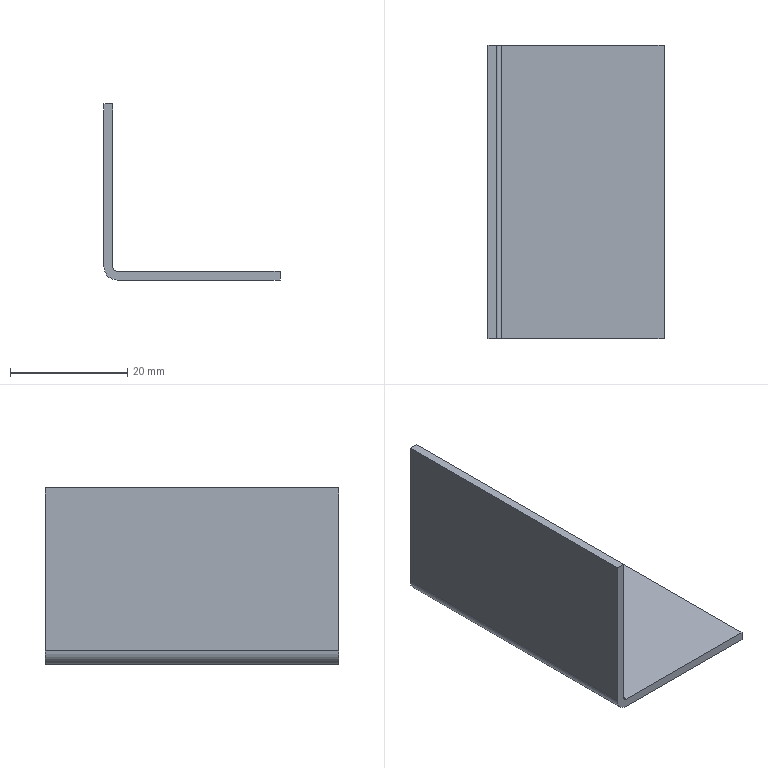Part | 1 solid | 10 faces | box 30 x 50 x 30 mm | volume 4340 mm3 | plane 8 | cylinder 2 | commonest cylinder face diameters 1.473 x1 4.473 x1
STEP:
#1=CARTESIAN_POINT('',(2.237,0.,-28.5));
#2=VERTEX_POINT('',#1);
#3=CARTESIAN_POINT('',(30.,0.,-28.5));
#4=VERTEX_POINT('',#3);
#5=CARTESIAN_POINT('',(0.,0.,-28.5));
#6=DIRECTION('',(1.,0.,0.));
#7=VECTOR('',#6,1000.);
#8=LINE('',#5,#7);
#9=EDGE_CURVE('',#2,#4,#8,.T.);
#10=ORIENTED_EDGE('',*,*,#9,.T.);
#11=CARTESIAN_POINT('',(30.,50.,-28.5));
#12=VERTEX_POINT('',#11);
#13=CARTESIAN_POINT('',(30.,50.,-28.5));
#14=DIRECTION('',(0.,-1.,0.));
#15=VECTOR('',#14,1000.);
#16=LINE('',#13,#15);
#17=EDGE_CURVE('',#12,#4,#16,.T.);
#18=ORIENTED_EDGE('',*,*,#17,.F.);
#19=CARTESIAN_POINT('',(2.237,50.,-28.5));
#20=VERTEX_POINT('',#19);
#21=CARTESIAN_POINT('',(0.,50.,-28.5));
#22=DIRECTION('',(1.,0.,0.));
#23=VECTOR('',#22,1000.);
#24=LINE('',#21,#23);
#25=EDGE_CURVE('',#20,#12,#24,.T.);
#26=ORIENTED_EDGE('',*,*,#25,.F.);
#27=CARTESIAN_POINT('',(2.237,50.,-28.5));
#28=DIRECTION('',(0.,-1.,0.));
#29=VECTOR('',#28,1000.);
#30=LINE('',#27,#29);
#31=EDGE_CURVE('',#20,#2,#30,.T.);
#32=ORIENTED_EDGE('',*,*,#31,.T.);
#33=EDGE_LOOP('',(#10,#18,#26,#32));
#34=FACE_OUTER_BOUND('',#33,.T.);
#35=CARTESIAN_POINT('',(0.,50.,-28.5));
#36=DIRECTION('',(0.,0.,-1.));
#37=DIRECTION('',(-1.,0.,0.));
#38=AXIS2_PLACEMENT_3D('',#35,#36,#37);
#39=PLANE('',#38);
#40=ADVANCED_FACE('',(#34),#39,.F.);
#41=CARTESIAN_POINT('',(30.,0.,-30.));
#42=VERTEX_POINT('',#41);
#43=CARTESIAN_POINT('',(30.,0.,-30.));
#44=DIRECTION('',(0.,0.,1.));
#45=VECTOR('',#44,1000.);
#46=LINE('',#43,#45);
#47=EDGE_CURVE('',#42,#4,#46,.T.);
#48=ORIENTED_EDGE('',*,*,#47,.F.);
#49=CARTESIAN_POINT('',(30.,50.,-30.));
#50=VERTEX_POINT('',#49);
#51=CARTESIAN_POINT('',(30.,50.,-30.));
#52=DIRECTION('',(0.,-1.,0.));
#53=VECTOR('',#52,1000.);
#54=LINE('',#51,#53);
#55=EDGE_CURVE('',#50,#42,#54,.T.);
#56=ORIENTED_EDGE('',*,*,#55,.F.);
#57=CARTESIAN_POINT('',(30.,50.,-30.));
#58=DIRECTION('',(0.,0.,1.));
#59=VECTOR('',#58,1000.);
#60=LINE('',#57,#59);
#61=EDGE_CURVE('',#50,#12,#60,.T.);
#62=ORIENTED_EDGE('',*,*,#61,.T.);
#63=ORIENTED_EDGE('',*,*,#17,.T.);
#64=EDGE_LOOP('',(#48,#56,#62,#63));
#65=FACE_OUTER_BOUND('',#64,.T.);
#66=CARTESIAN_POINT('',(30.,50.,-30.));
#67=DIRECTION('',(1.,0.,0.));
#68=DIRECTION('',(0.,0.,-1.));
#69=AXIS2_PLACEMENT_3D('',#66,#67,#68);
#70=PLANE('',#69);
#71=ADVANCED_FACE('',(#65),#70,.T.);
#72=CARTESIAN_POINT('',(2.237,0.,-30.));
#73=VERTEX_POINT('',#72);
#74=CARTESIAN_POINT('',(0.,0.,-30.));
#75=DIRECTION('',(1.,0.,0.));
#76=VECTOR('',#75,1000.);
#77=LINE('',#74,#76);
#78=EDGE_CURVE('',#73,#42,#77,.T.);
#79=ORIENTED_EDGE('',*,*,#78,.F.);
#80=CARTESIAN_POINT('',(2.237,50.,-30.));
#81=VERTEX_POINT('',#80);
#82=CARTESIAN_POINT('',(2.237,50.,-30.));
#83=DIRECTION('',(0.,-1.,0.));
#84=VECTOR('',#83,1000.);
#85=LINE('',#82,#84);
#86=EDGE_CURVE('',#81,#73,#85,.T.);
#87=ORIENTED_EDGE('',*,*,#86,.F.);
#88=CARTESIAN_POINT('',(0.,50.,-30.));
#89=DIRECTION('',(1.,0.,0.));
#90=VECTOR('',#89,1000.);
#91=LINE('',#88,#90);
#92=EDGE_CURVE('',#81,#50,#91,.T.);
#93=ORIENTED_EDGE('',*,*,#92,.T.);
#94=ORIENTED_EDGE('',*,*,#55,.T.);
#95=EDGE_LOOP('',(#79,#87,#93,#94));
#96=FACE_OUTER_BOUND('',#95,.T.);
#97=CARTESIAN_POINT('',(0.,50.,-30.));
#98=DIRECTION('',(0.,0.,-1.));
#99=DIRECTION('',(-1.,0.,0.));
#100=AXIS2_PLACEMENT_3D('',#97,#98,#99);
#101=PLANE('',#100);
#102=ADVANCED_FACE('',(#96),#101,.T.);
#103=CARTESIAN_POINT('',(0.,0.,-27.763));
#104=VERTEX_POINT('',#103);
#105=CARTESIAN_POINT('',(2.237,0.,-27.763));
#106=DIRECTION('',(0.,-1.,0.));
#107=DIRECTION('',(0.,0.,1.));
#108=AXIS2_PLACEMENT_3D('',#105,#106,#107);
#109=CIRCLE('',#108,2.237);
#110=EDGE_CURVE('',#104,#73,#109,.T.);
#111=ORIENTED_EDGE('',*,*,#110,.F.);
#112=CARTESIAN_POINT('',(0.,50.,-27.763));
#113=VERTEX_POINT('',#112);
#114=CARTESIAN_POINT('',(0.,50.,-27.763));
#115=DIRECTION('',(0.,-1.,0.));
#116=VECTOR('',#115,1000.);
#117=LINE('',#114,#116);
#118=EDGE_CURVE('',#113,#104,#117,.T.);
#119=ORIENTED_EDGE('',*,*,#118,.F.);
#120=CARTESIAN_POINT('',(2.237,50.,-27.763));
#121=DIRECTION('',(0.,-1.,0.));
#122=DIRECTION('',(0.,0.,1.));
#123=AXIS2_PLACEMENT_3D('',#120,#121,#122);
#124=CIRCLE('',#123,2.237);
#125=EDGE_CURVE('',#113,#81,#124,.T.);
#126=ORIENTED_EDGE('',*,*,#125,.T.);
#127=ORIENTED_EDGE('',*,*,#86,.T.);
#128=EDGE_LOOP('',(#111,#119,#126,#127));
#129=FACE_OUTER_BOUND('',#128,.T.);
#130=CARTESIAN_POINT('',(2.237,50.,-27.763));
#131=DIRECTION('',(0.,-1.,0.));
#132=DIRECTION('',(0.,0.,-1.));
#133=AXIS2_PLACEMENT_3D('',#130,#131,#132);
#134=CYLINDRICAL_SURFACE('',#133,2.237);
#135=ADVANCED_FACE('',(#129),#134,.T.);
#136=CARTESIAN_POINT('',(0.,0.,0.));
#137=VERTEX_POINT('',#136);
#138=CARTESIAN_POINT('',(0.,0.,-30.));
#139=DIRECTION('',(0.,0.,-1.));
#140=VECTOR('',#139,1000.);
#141=LINE('',#138,#140);
#142=EDGE_CURVE('',#137,#104,#141,.T.);
#143=ORIENTED_EDGE('',*,*,#142,.F.);
#144=CARTESIAN_POINT('',(0.,50.,0.));
#145=VERTEX_POINT('',#144);
#146=CARTESIAN_POINT('',(0.,50.,0.));
#147=DIRECTION('',(0.,-1.,0.));
#148=VECTOR('',#147,1000.);
#149=LINE('',#146,#148);
#150=EDGE_CURVE('',#145,#137,#149,.T.);
#151=ORIENTED_EDGE('',*,*,#150,.F.);
#152=CARTESIAN_POINT('',(0.,50.,-30.));
#153=DIRECTION('',(0.,0.,-1.));
#154=VECTOR('',#153,1000.);
#155=LINE('',#152,#154);
#156=EDGE_CURVE('',#145,#113,#155,.T.);
#157=ORIENTED_EDGE('',*,*,#156,.T.);
#158=ORIENTED_EDGE('',*,*,#118,.T.);
#159=EDGE_LOOP('',(#143,#151,#157,#158));
#160=FACE_OUTER_BOUND('',#159,.T.);
#161=CARTESIAN_POINT('',(0.,50.,-30.));
#162=DIRECTION('',(-1.,0.,0.));
#163=DIRECTION('',(0.,0.,1.));
#164=AXIS2_PLACEMENT_3D('',#161,#162,#163);
#165=PLANE('',#164);
#166=ADVANCED_FACE('',(#160),#165,.T.);
#167=CARTESIAN_POINT('',(1.5,0.,0.));
#168=VERTEX_POINT('',#167);
#169=CARTESIAN_POINT('',(1.5,0.,0.));
#170=DIRECTION('',(-1.,0.,0.));
#171=VECTOR('',#170,1000.);
#172=LINE('',#169,#171);
#173=EDGE_CURVE('',#168,#137,#172,.T.);
#174=ORIENTED_EDGE('',*,*,#173,.F.);
#175=CARTESIAN_POINT('',(1.5,50.,0.));
#176=VERTEX_POINT('',#175);
#177=CARTESIAN_POINT('',(1.5,50.,0.));
#178=DIRECTION('',(0.,-1.,0.));
#179=VECTOR('',#178,1000.);
#180=LINE('',#177,#179);
#181=EDGE_CURVE('',#176,#168,#180,.T.);
#182=ORIENTED_EDGE('',*,*,#181,.F.);
#183=CARTESIAN_POINT('',(1.5,50.,0.));
#184=DIRECTION('',(-1.,0.,0.));
#185=VECTOR('',#184,1000.);
#186=LINE('',#183,#185);
#187=EDGE_CURVE('',#176,#145,#186,.T.);
#188=ORIENTED_EDGE('',*,*,#187,.T.);
#189=ORIENTED_EDGE('',*,*,#150,.T.);
#190=EDGE_LOOP('',(#174,#182,#188,#189));
#191=FACE_OUTER_BOUND('',#190,.T.);
#192=CARTESIAN_POINT('',(1.5,50.,0.));
#193=DIRECTION('',(0.,0.,1.));
#194=DIRECTION('',(1.,0.,0.));
#195=AXIS2_PLACEMENT_3D('',#192,#193,#194);
#196=PLANE('',#195);
#197=ADVANCED_FACE('',(#191),#196,.T.);
#198=CARTESIAN_POINT('',(1.5,0.,-27.763));
#199=VERTEX_POINT('',#198);
#200=CARTESIAN_POINT('',(1.5,0.,-30.));
#201=DIRECTION('',(0.,0.,-1.));
#202=VECTOR('',#201,1000.);
#203=LINE('',#200,#202);
#204=EDGE_CURVE('',#168,#199,#203,.T.);
#205=ORIENTED_EDGE('',*,*,#204,.T.);
#206=CARTESIAN_POINT('',(1.5,50.,-27.763));
#207=VERTEX_POINT('',#206);
#208=CARTESIAN_POINT('',(1.5,50.,-27.763));
#209=DIRECTION('',(0.,-1.,0.));
#210=VECTOR('',#209,1000.);
#211=LINE('',#208,#210);
#212=EDGE_CURVE('',#207,#199,#211,.T.);
#213=ORIENTED_EDGE('',*,*,#212,.F.);
#214=CARTESIAN_POINT('',(1.5,50.,-30.));
#215=DIRECTION('',(0.,0.,-1.));
#216=VECTOR('',#215,1000.);
#217=LINE('',#214,#216);
#218=EDGE_CURVE('',#176,#207,#217,.T.);
#219=ORIENTED_EDGE('',*,*,#218,.F.);
#220=ORIENTED_EDGE('',*,*,#181,.T.);
#221=EDGE_LOOP('',(#205,#213,#219,#220));
#222=FACE_OUTER_BOUND('',#221,.T.);
#223=CARTESIAN_POINT('',(1.5,50.,-30.));
#224=DIRECTION('',(-1.,0.,0.));
#225=DIRECTION('',(0.,0.,1.));
#226=AXIS2_PLACEMENT_3D('',#223,#224,#225);
#227=PLANE('',#226);
#228=ADVANCED_FACE('',(#222),#227,.F.);
#229=CARTESIAN_POINT('',(2.237,0.,-27.763));
#230=DIRECTION('',(0.,-1.,0.));
#231=DIRECTION('',(1.,0.,0.));
#232=AXIS2_PLACEMENT_3D('',#229,#230,#231);
#233=CIRCLE('',#232,0.7366);
#234=EDGE_CURVE('',#199,#2,#233,.T.);
#235=ORIENTED_EDGE('',*,*,#234,.T.);
#236=ORIENTED_EDGE('',*,*,#31,.F.);
#237=CARTESIAN_POINT('',(2.237,50.,-27.763));
#238=DIRECTION('',(0.,-1.,0.));
#239=DIRECTION('',(1.,0.,0.));
#240=AXIS2_PLACEMENT_3D('',#237,#238,#239);
#241=CIRCLE('',#240,0.7366);
#242=EDGE_CURVE('',#207,#20,#241,.T.);
#243=ORIENTED_EDGE('',*,*,#242,.F.);
#244=ORIENTED_EDGE('',*,*,#212,.T.);
#245=EDGE_LOOP('',(#235,#236,#243,#244));
#246=FACE_OUTER_BOUND('',#245,.T.);
#247=CARTESIAN_POINT('',(2.237,50.,-27.763));
#248=DIRECTION('',(0.,-1.,0.));
#249=DIRECTION('',(0.,0.,-1.));
#250=AXIS2_PLACEMENT_3D('',#247,#248,#249);
#251=CYLINDRICAL_SURFACE('',#250,0.7366);
#252=ADVANCED_FACE('',(#246),#251,.F.);
#253=ORIENTED_EDGE('',*,*,#218,.T.);
#254=ORIENTED_EDGE('',*,*,#242,.T.);
#255=ORIENTED_EDGE('',*,*,#25,.T.);
#256=ORIENTED_EDGE('',*,*,#61,.F.);
#257=ORIENTED_EDGE('',*,*,#92,.F.);
#258=ORIENTED_EDGE('',*,*,#125,.F.);
#259=ORIENTED_EDGE('',*,*,#156,.F.);
#260=ORIENTED_EDGE('',*,*,#187,.F.);
#261=EDGE_LOOP('',(#253,#254,#255,#256,#257,#258,#259,#260));
#262=FACE_OUTER_BOUND('',#261,.T.);
#263=CARTESIAN_POINT('',(2.237,50.,-27.763));
#264=DIRECTION('',(0.,1.,0.));
#265=DIRECTION('',(1.,0.,0.));
#266=AXIS2_PLACEMENT_3D('',#263,#264,#265);
#267=PLANE('',#266);
#268=ADVANCED_FACE('',(#262),#267,.T.);
#269=ORIENTED_EDGE('',*,*,#9,.F.);
#270=ORIENTED_EDGE('',*,*,#234,.F.);
#271=ORIENTED_EDGE('',*,*,#204,.F.);
#272=ORIENTED_EDGE('',*,*,#173,.T.);
#273=ORIENTED_EDGE('',*,*,#142,.T.);
#274=ORIENTED_EDGE('',*,*,#110,.T.);
#275=ORIENTED_EDGE('',*,*,#78,.T.);
#276=ORIENTED_EDGE('',*,*,#47,.T.);
#277=EDGE_LOOP('',(#269,#270,#271,#272,#273,#274,#275,#276));
#278=FACE_OUTER_BOUND('',#277,.T.);
#279=CARTESIAN_POINT('',(2.237,0.,-27.763));
#280=DIRECTION('',(0.,1.,0.));
#281=DIRECTION('',(1.,0.,0.));
#282=AXIS2_PLACEMENT_3D('',#279,#280,#281);
#283=PLANE('',#282);
#284=ADVANCED_FACE('',(#278),#283,.F.);
#285=CLOSED_SHELL('',(#40,#71,#102,#135,#166,#197,#228,#252,#268,#284));
#286=MANIFOLD_SOLID_BREP('',#285);
#287=CARTESIAN_POINT('',(0.,0.,0.));
#288=DIRECTION('',(0.,0.,1.));
#289=DIRECTION('',(1.,0.,0.));
#290=AXIS2_PLACEMENT_3D('',#287,#288,#289);
#291=(LENGTH_UNIT()NAMED_UNIT(*)SI_UNIT(.MILLI.,.METRE.));
#292=UNCERTAINTY_MEASURE_WITH_UNIT(LENGTH_MEASURE(0.00001),#291,'','');
#293=(NAMED_UNIT(*)PLANE_ANGLE_UNIT()SI_UNIT($,.RADIAN.));
#294=(NAMED_UNIT(*)SI_UNIT($,.STERADIAN.)SOLID_ANGLE_UNIT());
#295=(GEOMETRIC_REPRESENTATION_CONTEXT(3)GLOBAL_UNCERTAINTY_ASSIGNED_CONTEXT((#292))GLOBAL_UNIT_ASSIGNED_CONTEXT((#291,#293,#294))REPRESENTATION_CONTEXT('',''));
#296=ADVANCED_BREP_SHAPE_REPRESENTATION('',(#286,#290),#295);